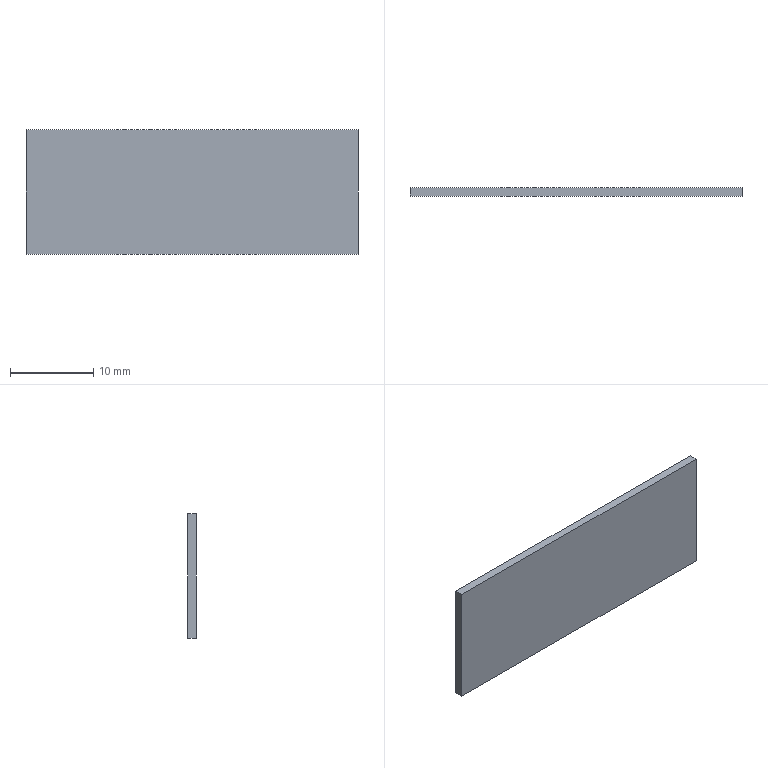Part | SolidWorks | features Extrusion 1 | 1 solid | 6 faces | box 40 x 1 x 15 mm | volume 600 mm3 | plane 6
STEP:
#1=CARTESIAN_POINT('',(20.,0.,7.5));
#2=VERTEX_POINT('',#1);
#3=CARTESIAN_POINT('',(20.,0.,-7.5));
#4=VERTEX_POINT('',#3);
#5=CARTESIAN_POINT('',(20.,0.,7.5));
#6=DIRECTION('',(0.,0.,-1.));
#7=VECTOR('',#6,1000.);
#8=LINE('',#5,#7);
#9=EDGE_CURVE('',#2,#4,#8,.T.);
#10=ORIENTED_EDGE('',*,*,#9,.T.);
#11=CARTESIAN_POINT('',(20.,1.,-7.5));
#12=VERTEX_POINT('',#11);
#13=CARTESIAN_POINT('',(20.,1.,-7.5));
#14=DIRECTION('',(0.,-1.,0.));
#15=VECTOR('',#14,1000.);
#16=LINE('',#13,#15);
#17=EDGE_CURVE('',#12,#4,#16,.T.);
#18=ORIENTED_EDGE('',*,*,#17,.F.);
#19=CARTESIAN_POINT('',(20.,1.,7.5));
#20=VERTEX_POINT('',#19);
#21=CARTESIAN_POINT('',(20.,1.,7.5));
#22=DIRECTION('',(0.,0.,-1.));
#23=VECTOR('',#22,1000.);
#24=LINE('',#21,#23);
#25=EDGE_CURVE('',#20,#12,#24,.T.);
#26=ORIENTED_EDGE('',*,*,#25,.F.);
#27=CARTESIAN_POINT('',(20.,1.,7.5));
#28=DIRECTION('',(0.,-1.,0.));
#29=VECTOR('',#28,1000.);
#30=LINE('',#27,#29);
#31=EDGE_CURVE('',#20,#2,#30,.T.);
#32=ORIENTED_EDGE('',*,*,#31,.T.);
#33=EDGE_LOOP('',(#10,#18,#26,#32));
#34=FACE_OUTER_BOUND('',#33,.T.);
#35=CARTESIAN_POINT('',(20.,1.,7.5));
#36=DIRECTION('',(-1.,0.,0.));
#37=DIRECTION('',(0.,0.,1.));
#38=AXIS2_PLACEMENT_3D('',#35,#36,#37);
#39=PLANE('',#38);
#40=ADVANCED_FACE('',(#34),#39,.F.);
#41=CARTESIAN_POINT('',(-20.,0.,-7.5));
#42=VERTEX_POINT('',#41);
#43=CARTESIAN_POINT('',(-20.,0.,-7.5));
#44=DIRECTION('',(-1.,0.,0.));
#45=VECTOR('',#44,1000.);
#46=LINE('',#43,#45);
#47=EDGE_CURVE('',#4,#42,#46,.T.);
#48=ORIENTED_EDGE('',*,*,#47,.T.);
#49=CARTESIAN_POINT('',(-20.,1.,-7.5));
#50=VERTEX_POINT('',#49);
#51=CARTESIAN_POINT('',(-20.,1.,-7.5));
#52=DIRECTION('',(0.,-1.,0.));
#53=VECTOR('',#52,1000.);
#54=LINE('',#51,#53);
#55=EDGE_CURVE('',#50,#42,#54,.T.);
#56=ORIENTED_EDGE('',*,*,#55,.F.);
#57=CARTESIAN_POINT('',(-20.,1.,-7.5));
#58=DIRECTION('',(-1.,0.,0.));
#59=VECTOR('',#58,1000.);
#60=LINE('',#57,#59);
#61=EDGE_CURVE('',#12,#50,#60,.T.);
#62=ORIENTED_EDGE('',*,*,#61,.F.);
#63=ORIENTED_EDGE('',*,*,#17,.T.);
#64=EDGE_LOOP('',(#48,#56,#62,#63));
#65=FACE_OUTER_BOUND('',#64,.T.);
#66=CARTESIAN_POINT('',(-20.,1.,-7.5));
#67=DIRECTION('',(0.,0.,1.));
#68=DIRECTION('',(1.,0.,0.));
#69=AXIS2_PLACEMENT_3D('',#66,#67,#68);
#70=PLANE('',#69);
#71=ADVANCED_FACE('',(#65),#70,.F.);
#72=CARTESIAN_POINT('',(-20.,0.,7.5));
#73=VERTEX_POINT('',#72);
#74=CARTESIAN_POINT('',(-20.,0.,7.5));
#75=DIRECTION('',(0.,0.,1.));
#76=VECTOR('',#75,1000.);
#77=LINE('',#74,#76);
#78=EDGE_CURVE('',#42,#73,#77,.T.);
#79=ORIENTED_EDGE('',*,*,#78,.T.);
#80=CARTESIAN_POINT('',(-20.,1.,7.5));
#81=VERTEX_POINT('',#80);
#82=CARTESIAN_POINT('',(-20.,1.,7.5));
#83=DIRECTION('',(0.,-1.,0.));
#84=VECTOR('',#83,1000.);
#85=LINE('',#82,#84);
#86=EDGE_CURVE('',#81,#73,#85,.T.);
#87=ORIENTED_EDGE('',*,*,#86,.F.);
#88=CARTESIAN_POINT('',(-20.,1.,7.5));
#89=DIRECTION('',(0.,0.,1.));
#90=VECTOR('',#89,1000.);
#91=LINE('',#88,#90);
#92=EDGE_CURVE('',#50,#81,#91,.T.);
#93=ORIENTED_EDGE('',*,*,#92,.F.);
#94=ORIENTED_EDGE('',*,*,#55,.T.);
#95=EDGE_LOOP('',(#79,#87,#93,#94));
#96=FACE_OUTER_BOUND('',#95,.T.);
#97=CARTESIAN_POINT('',(-20.,1.,7.5));
#98=DIRECTION('',(1.,0.,0.));
#99=DIRECTION('',(0.,0.,-1.));
#100=AXIS2_PLACEMENT_3D('',#97,#98,#99);
#101=PLANE('',#100);
#102=ADVANCED_FACE('',(#96),#101,.F.);
#103=CARTESIAN_POINT('',(-20.,0.,7.5));
#104=DIRECTION('',(1.,0.,0.));
#105=VECTOR('',#104,1000.);
#106=LINE('',#103,#105);
#107=EDGE_CURVE('',#73,#2,#106,.T.);
#108=ORIENTED_EDGE('',*,*,#107,.T.);
#109=ORIENTED_EDGE('',*,*,#31,.F.);
#110=CARTESIAN_POINT('',(-20.,1.,7.5));
#111=DIRECTION('',(1.,0.,0.));
#112=VECTOR('',#111,1000.);
#113=LINE('',#110,#112);
#114=EDGE_CURVE('',#81,#20,#113,.T.);
#115=ORIENTED_EDGE('',*,*,#114,.F.);
#116=ORIENTED_EDGE('',*,*,#86,.T.);
#117=EDGE_LOOP('',(#108,#109,#115,#116));
#118=FACE_OUTER_BOUND('',#117,.T.);
#119=CARTESIAN_POINT('',(-20.,1.,7.5));
#120=DIRECTION('',(0.,0.,-1.));
#121=DIRECTION('',(-1.,0.,0.));
#122=AXIS2_PLACEMENT_3D('',#119,#120,#121);
#123=PLANE('',#122);
#124=ADVANCED_FACE('',(#118),#123,.F.);
#125=ORIENTED_EDGE('',*,*,#25,.T.);
#126=ORIENTED_EDGE('',*,*,#61,.T.);
#127=ORIENTED_EDGE('',*,*,#92,.T.);
#128=ORIENTED_EDGE('',*,*,#114,.T.);
#129=EDGE_LOOP('',(#125,#126,#127,#128));
#130=FACE_OUTER_BOUND('',#129,.T.);
#131=CARTESIAN_POINT('',(0.,1.,0.));
#132=DIRECTION('',(0.,-1.,0.));
#133=DIRECTION('',(0.,0.,-1.));
#134=AXIS2_PLACEMENT_3D('',#131,#132,#133);
#135=PLANE('',#134);
#136=ADVANCED_FACE('',(#130),#135,.F.);
#137=ORIENTED_EDGE('',*,*,#9,.F.);
#138=ORIENTED_EDGE('',*,*,#107,.F.);
#139=ORIENTED_EDGE('',*,*,#78,.F.);
#140=ORIENTED_EDGE('',*,*,#47,.F.);
#141=EDGE_LOOP('',(#137,#138,#139,#140));
#142=FACE_OUTER_BOUND('',#141,.T.);
#143=CARTESIAN_POINT('',(0.,0.,0.));
#144=DIRECTION('',(0.,-1.,0.));
#145=DIRECTION('',(0.,0.,-1.));
#146=AXIS2_PLACEMENT_3D('',#143,#144,#145);
#147=PLANE('',#146);
#148=ADVANCED_FACE('',(#142),#147,.T.);
#149=CLOSED_SHELL('',(#40,#71,#102,#124,#136,#148));
#150=MANIFOLD_SOLID_BREP('',#149);
#151=CARTESIAN_POINT('',(0.,0.,0.));
#152=DIRECTION('',(0.,0.,1.));
#153=DIRECTION('',(1.,0.,0.));
#154=AXIS2_PLACEMENT_3D('',#151,#152,#153);
#155=(LENGTH_UNIT()NAMED_UNIT(*)SI_UNIT(.MILLI.,.METRE.));
#156=UNCERTAINTY_MEASURE_WITH_UNIT(LENGTH_MEASURE(0.00001),#155,'','');
#157=(NAMED_UNIT(*)PLANE_ANGLE_UNIT()SI_UNIT($,.RADIAN.));
#158=(NAMED_UNIT(*)SI_UNIT($,.STERADIAN.)SOLID_ANGLE_UNIT());
#159=(GEOMETRIC_REPRESENTATION_CONTEXT(3)GLOBAL_UNCERTAINTY_ASSIGNED_CONTEXT((#156))GLOBAL_UNIT_ASSIGNED_CONTEXT((#155,#157,#158))REPRESENTATION_CONTEXT('',''));
#160=ADVANCED_BREP_SHAPE_REPRESENTATION('',(#150,#154),#159);